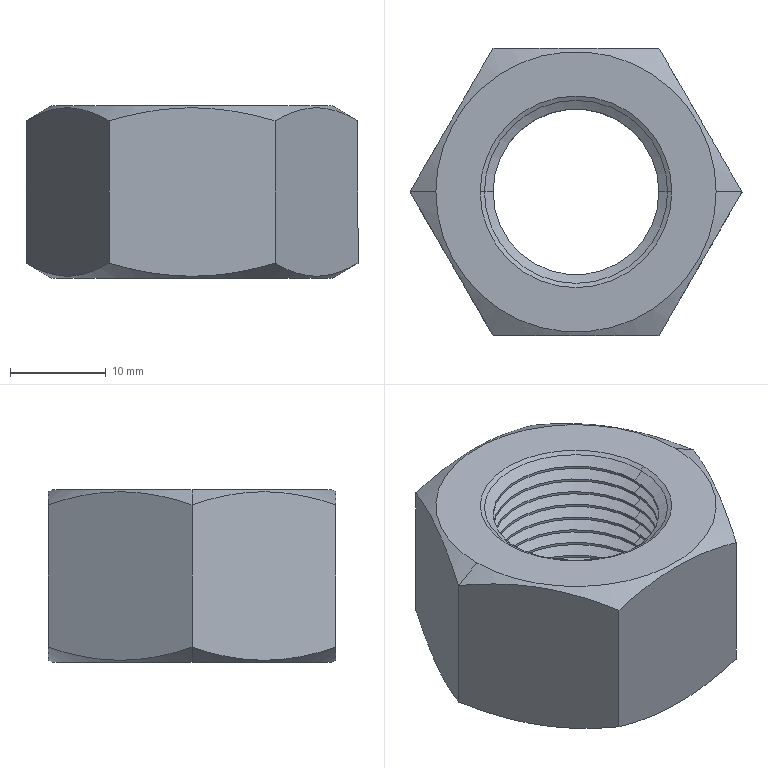Part | STEP file | hex nuts, style 1-grades ab gb_GB_FASTENER_NUT_SNAB1  B M20-S | 1 solid | 80 faces | box 34.641 x 30 x 18 mm | volume 9181 mm3 | cone 52 | cylinder 20 | plane 8 | commonest cylinder face diameters 17.294 x20